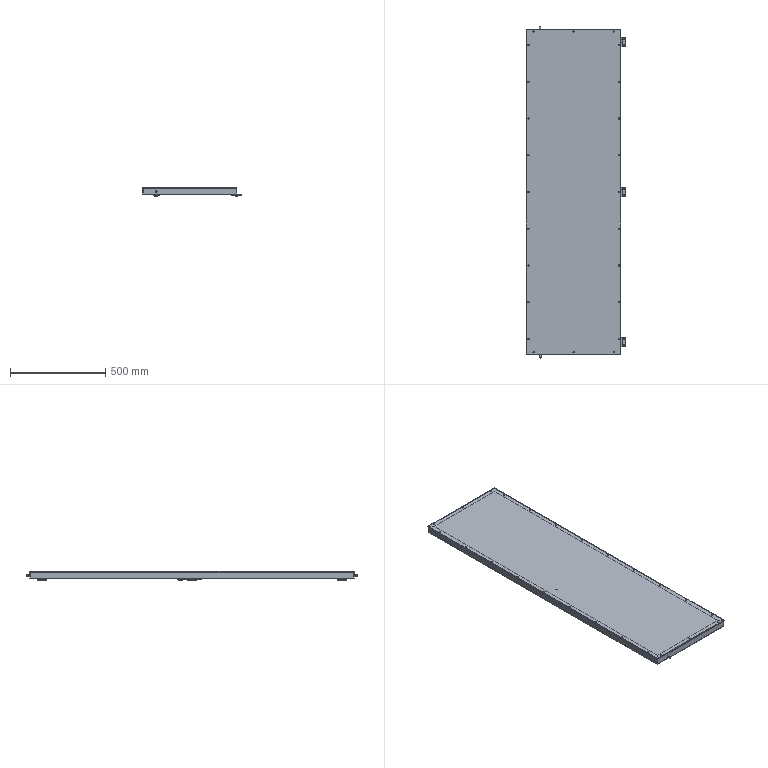Part | SolidWorks | 13 solids | 1434 faces | box 519.5 x 1742 x 50.5 mm | volume 4569097 mm3 | cylinder 623 | plane 564 | spline 194 | cone 53 | commonest cylinder face diameters 1 x144 5 x66 0.8 x52 6.5 x48 6.1 x46 6 x32